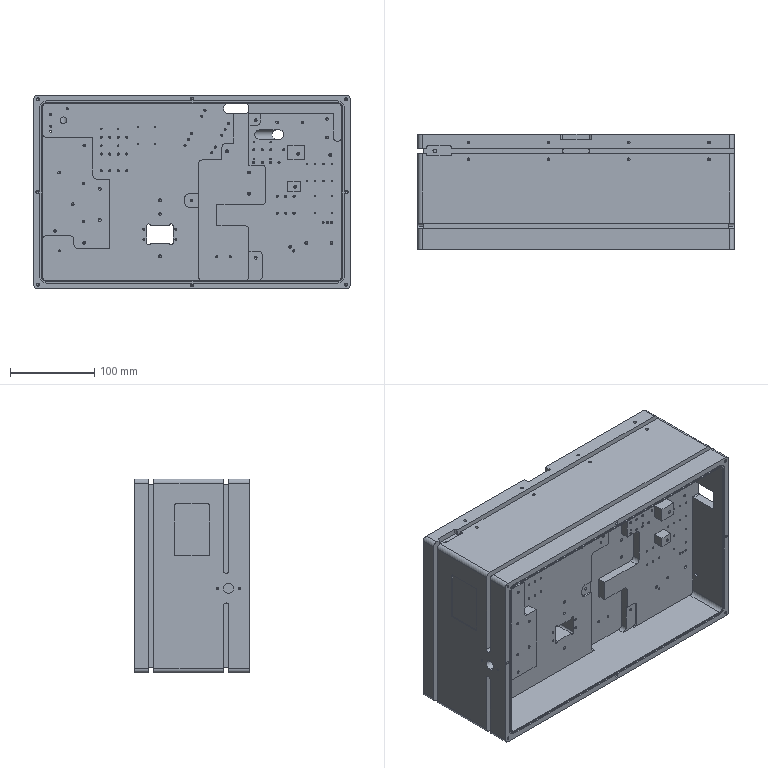Part | SolidWorks | features ICE 36, HoleWzd 21, Fillet 12, Extrusion 1, SweepCut 1 | 1 solid | 1139 faces | box 375 x 137 x 230 mm | volume 4002345 mm3 | cylinder 541 | cone 386 | plane 206 | torus 6 | commonest cylinder face diameters 2.5 x156 3.3 x144 10 x97 1.6 x48 3 x20 4 x20